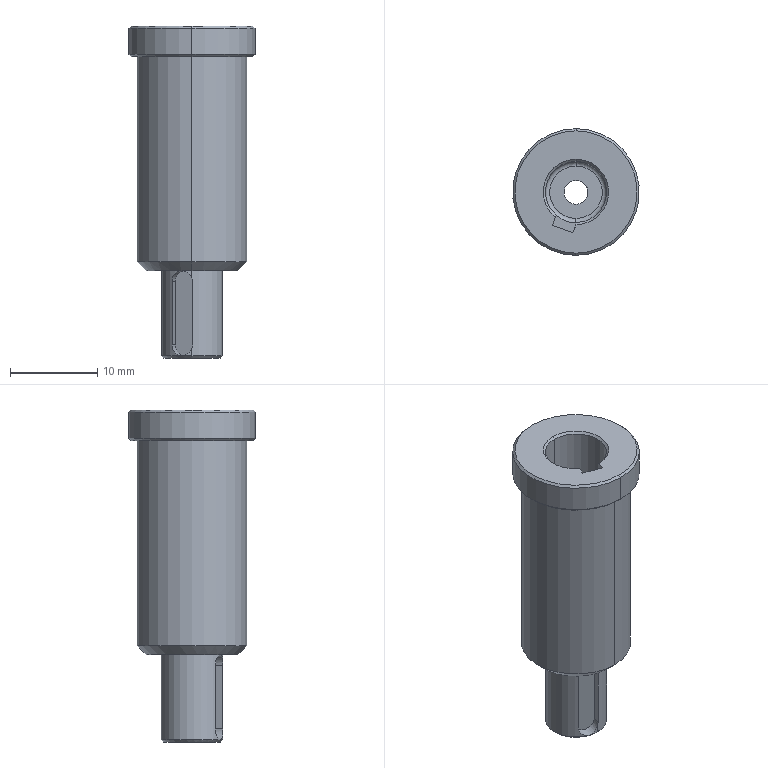Part | STEP file | 2026.6.15-Main Assembly图.sldasm-Part-156 | 1 solid | 41 faces | box 14.5 x 14.5 x 38 mm | volume 3109 mm3 | cylinder 14 | cone 13 | plane 12 | torus 2 | commonest cylinder face diameters 7 x6 2.5 x2 2.75 x2 12.5 x2 14.5 x2
STEP:
#1=CARTESIAN_POINT('',(-1571.41,1398.006,3694.571));
#2=VERTEX_POINT('',#1);
#3=CARTESIAN_POINT('',(-1571.418,1387.506,3694.571));
#4=VERTEX_POINT('',#3);
#5=CARTESIAN_POINT('',(-1571.414,1392.756,3694.571));
#6=DIRECTION('',(0.,0.,-1.));
#7=DIRECTION('',(0.0007664,1.,0.));
#8=AXIS2_PLACEMENT_3D('',#5,#6,#7);
#9=CIRCLE('',#8,5.25);
#10=EDGE_CURVE('',#2,#4,#9,.T.);
#11=ORIENTED_EDGE('',*,*,#10,.F.);
#12=CARTESIAN_POINT('',(-1571.409,1399.006,3695.571));
#13=VERTEX_POINT('',#12);
#14=CARTESIAN_POINT('',(-1571.41,1398.006,3694.571));
#15=DIRECTION('',(0.000542,0.7071,0.7071));
#16=VECTOR('',#15,1000.);
#17=LINE('',#14,#16);
#18=EDGE_CURVE('',#2,#13,#17,.T.);
#19=ORIENTED_EDGE('',*,*,#18,.T.);
#20=CARTESIAN_POINT('',(-1571.419,1386.506,3695.571));
#21=VERTEX_POINT('',#20);
#22=CARTESIAN_POINT('',(-1571.414,1392.756,3695.571));
#23=DIRECTION('',(0.,0.,1.));
#24=DIRECTION('',(0.0007664,1.,0.));
#25=AXIS2_PLACEMENT_3D('',#22,#23,#24);
#26=CIRCLE('',#25,6.25);
#27=EDGE_CURVE('',#21,#13,#26,.T.);
#28=ORIENTED_EDGE('',*,*,#27,.F.);
#29=CARTESIAN_POINT('',(-1571.418,1387.506,3694.571));
#30=DIRECTION('',(-0.000542,-0.7071,0.7071));
#31=VECTOR('',#30,1000.);
#32=LINE('',#29,#31);
#33=EDGE_CURVE('',#4,#21,#32,.T.);
#34=ORIENTED_EDGE('',*,*,#33,.F.);
#35=EDGE_LOOP('',(#11,#19,#28,#34));
#36=FACE_OUTER_BOUND('',#35,.T.);
#37=CARTESIAN_POINT('',(-1571.414,1392.756,3694.571));
#38=DIRECTION('',(0.,0.,1.));
#39=DIRECTION('',(-0.0007664,-1.,0.));
#40=AXIS2_PLACEMENT_3D('',#37,#38,#39);
#41=CONICAL_SURFACE('',#40,5.25,0.7854);
#42=ADVANCED_FACE('',(#36),#41,.T.);
#43=CARTESIAN_POINT('',(-1571.412,1396.006,3684.571));
#44=VERTEX_POINT('',#43);
#45=CARTESIAN_POINT('',(-1571.417,1389.506,3684.571));
#46=VERTEX_POINT('',#45);
#47=CARTESIAN_POINT('',(-1571.414,1392.756,3684.571));
#48=DIRECTION('',(0.,0.,-1.));
#49=DIRECTION('',(0.0007664,1.,0.));
#50=AXIS2_PLACEMENT_3D('',#47,#48,#49);
#51=CIRCLE('',#50,3.25);
#52=EDGE_CURVE('',#44,#46,#51,.T.);
#53=ORIENTED_EDGE('',*,*,#52,.F.);
#54=CARTESIAN_POINT('',(-1571.411,1396.256,3684.821));
#55=VERTEX_POINT('',#54);
#56=CARTESIAN_POINT('',(-1571.412,1396.006,3684.571));
#57=DIRECTION('',(0.000542,0.7071,0.7071));
#58=VECTOR('',#57,1000.);
#59=LINE('',#56,#58);
#60=EDGE_CURVE('',#44,#55,#59,.T.);
#61=ORIENTED_EDGE('',*,*,#60,.T.);
#62=CARTESIAN_POINT('',(-1571.417,1389.256,3684.821));
#63=VERTEX_POINT('',#62);
#64=CARTESIAN_POINT('',(-1571.414,1392.756,3684.821));
#65=DIRECTION('',(0.,0.,1.));
#66=DIRECTION('',(0.0007664,1.,0.));
#67=AXIS2_PLACEMENT_3D('',#64,#65,#66);
#68=CIRCLE('',#67,3.5);
#69=EDGE_CURVE('',#63,#55,#68,.T.);
#70=ORIENTED_EDGE('',*,*,#69,.F.);
#71=CARTESIAN_POINT('',(-1571.417,1389.506,3684.571));
#72=DIRECTION('',(-0.000542,-0.7071,0.7071));
#73=VECTOR('',#72,1000.);
#74=LINE('',#71,#73);
#75=EDGE_CURVE('',#46,#63,#74,.T.);
#76=ORIENTED_EDGE('',*,*,#75,.F.);
#77=EDGE_LOOP('',(#53,#61,#70,#76));
#78=FACE_OUTER_BOUND('',#77,.T.);
#79=CARTESIAN_POINT('',(-1571.414,1392.756,3684.571));
#80=DIRECTION('',(0.,0.,1.));
#81=DIRECTION('',(-0.0007664,-1.,0.));
#82=AXIS2_PLACEMENT_3D('',#79,#80,#81);
#83=CONICAL_SURFACE('',#82,3.25,0.7854);
#84=ADVANCED_FACE('',(#78),#83,.T.);
#85=CARTESIAN_POINT('',(-1571.415,1391.381,3684.821));
#86=VERTEX_POINT('',#85);
#87=CARTESIAN_POINT('',(-1571.413,1394.131,3684.821));
#88=VERTEX_POINT('',#87);
#89=CARTESIAN_POINT('',(-1571.414,1392.756,3684.821));
#90=DIRECTION('',(0.,0.,-1.));
#91=DIRECTION('',(0.0007664,1.,0.));
#92=AXIS2_PLACEMENT_3D('',#89,#90,#91);
#93=CIRCLE('',#92,1.375);
#94=EDGE_CURVE('',#86,#88,#93,.T.);
#95=ORIENTED_EDGE('',*,*,#94,.F.);
#96=CARTESIAN_POINT('',(-1571.415,1391.131,3684.571));
#97=VERTEX_POINT('',#96);
#98=CARTESIAN_POINT('',(-1571.415,1391.131,3684.571));
#99=DIRECTION('',(-0.000542,-0.7071,-0.7071));
#100=VECTOR('',#99,1000.);
#101=LINE('',#98,#100);
#102=EDGE_CURVE('',#86,#97,#101,.T.);
#103=ORIENTED_EDGE('',*,*,#102,.T.);
#104=CARTESIAN_POINT('',(-1571.413,1394.381,3684.571));
#105=VERTEX_POINT('',#104);
#106=CARTESIAN_POINT('',(-1571.414,1392.756,3684.571));
#107=DIRECTION('',(0.,0.,1.));
#108=DIRECTION('',(0.0007664,1.,0.));
#109=AXIS2_PLACEMENT_3D('',#106,#107,#108);
#110=CIRCLE('',#109,1.625);
#111=EDGE_CURVE('',#105,#97,#110,.T.);
#112=ORIENTED_EDGE('',*,*,#111,.F.);
#113=CARTESIAN_POINT('',(-1571.413,1394.381,3684.571));
#114=DIRECTION('',(0.000542,0.7071,-0.7071));
#115=VECTOR('',#114,1000.);
#116=LINE('',#113,#115);
#117=EDGE_CURVE('',#88,#105,#116,.T.);
#118=ORIENTED_EDGE('',*,*,#117,.F.);
#119=EDGE_LOOP('',(#95,#103,#112,#118));
#120=FACE_OUTER_BOUND('',#119,.T.);
#121=CARTESIAN_POINT('',(-1571.414,1392.756,3684.571));
#122=DIRECTION('',(0.,0.,-1.));
#123=DIRECTION('',(0.0007664,1.,0.));
#124=AXIS2_PLACEMENT_3D('',#121,#122,#123);
#125=CONICAL_SURFACE('',#124,1.625,0.7854);
#126=ADVANCED_FACE('',(#120),#125,.F.);
#127=CARTESIAN_POINT('',(-1571.411,1396.256,3722.321));
#128=VERTEX_POINT('',#127);
#129=CARTESIAN_POINT('',(-1573.696,1390.103,3722.321));
#130=VERTEX_POINT('',#129);
#131=CARTESIAN_POINT('',(-1571.414,1392.756,3722.321));
#132=DIRECTION('',(0.,0.,1.));
#133=DIRECTION('',(0.0007664,1.,0.));
#134=AXIS2_PLACEMENT_3D('',#131,#132,#133);
#135=CIRCLE('',#134,3.5);
#136=EDGE_CURVE('',#128,#130,#135,.T.);
#137=ORIENTED_EDGE('',*,*,#136,.F.);
#138=CARTESIAN_POINT('',(-1571.411,1396.506,3722.571));
#139=VERTEX_POINT('',#138);
#140=CARTESIAN_POINT('',(-1571.411,1396.506,3722.571));
#141=DIRECTION('',(0.000542,0.7071,0.7071));
#142=VECTOR('',#141,1000.);
#143=LINE('',#140,#142);
#144=EDGE_CURVE('',#128,#139,#143,.T.);
#145=ORIENTED_EDGE('',*,*,#144,.T.);
#146=CARTESIAN_POINT('',(-1573.787,1389.852,3722.571));
#147=VERTEX_POINT('',#146);
#148=CARTESIAN_POINT('',(-1571.414,1392.756,3722.571));
#149=DIRECTION('',(0.,0.,-1.));
#150=DIRECTION('',(0.0007664,1.,0.));
#151=AXIS2_PLACEMENT_3D('',#148,#149,#150);
#152=CIRCLE('',#151,3.75);
#153=EDGE_CURVE('',#147,#139,#152,.T.);
#154=ORIENTED_EDGE('',*,*,#153,.F.);
#155=CARTESIAN_POINT('',(-1573.696,1390.103,3722.321));
#156=CARTESIAN_POINT('',(-1573.727,1390.019,3722.404));
#157=CARTESIAN_POINT('',(-1573.757,1389.936,3722.487));
#158=CARTESIAN_POINT('',(-1573.787,1389.852,3722.571));
#159=B_SPLINE_CURVE_WITH_KNOTS('',3,(#155,#156,#157,#158),.UNSPECIFIED.,.F.,.F.,(4,4),(0.,0.0003653),.UNSPECIFIED.);
#160=EDGE_CURVE('',#130,#147,#159,.T.);
#161=ORIENTED_EDGE('',*,*,#160,.F.);
#162=EDGE_LOOP('',(#137,#145,#154,#161));
#163=FACE_OUTER_BOUND('',#162,.T.);
#164=CARTESIAN_POINT('',(-1571.414,1392.756,3722.571));
#165=DIRECTION('',(0.,0.,1.));
#166=DIRECTION('',(-0.0007664,-1.,0.));
#167=AXIS2_PLACEMENT_3D('',#164,#165,#166);
#168=CONICAL_SURFACE('',#167,3.75,0.7854);
#169=ADVANCED_FACE('',(#163),#168,.F.);
#170=ORIENTED_EDGE('',*,*,#144,.F.);
#171=CARTESIAN_POINT('',(-1571.344,1389.257,3722.321));
#172=VERTEX_POINT('',#171);
#173=CARTESIAN_POINT('',(-1571.414,1392.756,3722.321));
#174=DIRECTION('',(0.,0.,1.));
#175=DIRECTION('',(0.0007664,1.,0.));
#176=AXIS2_PLACEMENT_3D('',#173,#174,#175);
#177=CIRCLE('',#176,3.5);
#178=EDGE_CURVE('',#172,#128,#177,.T.);
#179=ORIENTED_EDGE('',*,*,#178,.F.);
#180=CARTESIAN_POINT('',(-1571.417,1389.054,3722.524));
#181=VERTEX_POINT('',#180);
#182=CARTESIAN_POINT('',(-1571.417,1389.054,3722.524));
#183=CARTESIAN_POINT('',(-1571.393,1389.121,3722.456));
#184=CARTESIAN_POINT('',(-1571.368,1389.189,3722.388));
#185=CARTESIAN_POINT('',(-1571.344,1389.257,3722.321));
#186=B_SPLINE_CURVE_WITH_KNOTS('',3,(#182,#183,#184,#185),.UNSPECIFIED.,.F.,.F.,(4,4),(0.00006889,0.0003653),.UNSPECIFIED.);
#187=EDGE_CURVE('',#181,#172,#186,.T.);
#188=ORIENTED_EDGE('',*,*,#187,.F.);
#189=CARTESIAN_POINT('',(-1571.417,1389.006,3722.571));
#190=VERTEX_POINT('',#189);
#191=CARTESIAN_POINT('',(-1571.417,1389.006,3722.571));
#192=DIRECTION('',(-0.000542,-0.7071,0.7071));
#193=VECTOR('',#192,1000.);
#194=LINE('',#191,#193);
#195=EDGE_CURVE('',#181,#190,#194,.T.);
#196=ORIENTED_EDGE('',*,*,#195,.T.);
#197=CARTESIAN_POINT('',(-1571.414,1392.756,3722.571));
#198=DIRECTION('',(0.,0.,-1.));
#199=DIRECTION('',(0.0007664,1.,0.));
#200=AXIS2_PLACEMENT_3D('',#197,#198,#199);
#201=CIRCLE('',#200,3.75);
#202=EDGE_CURVE('',#139,#190,#201,.T.);
#203=ORIENTED_EDGE('',*,*,#202,.F.);
#204=EDGE_LOOP('',(#170,#179,#188,#196,#203));
#205=FACE_OUTER_BOUND('',#204,.T.);
#206=CARTESIAN_POINT('',(-1571.414,1392.756,3722.571));
#207=DIRECTION('',(0.,0.,1.));
#208=DIRECTION('',(-0.0007664,-1.,0.));
#209=AXIS2_PLACEMENT_3D('',#206,#207,#208);
#210=CONICAL_SURFACE('',#209,3.75,0.7854);
#211=ADVANCED_FACE('',(#205),#210,.F.);
#212=CARTESIAN_POINT('',(-1571.419,1385.756,3722.571));
#213=VERTEX_POINT('',#212);
#214=CARTESIAN_POINT('',(-1571.409,1399.756,3722.571));
#215=VERTEX_POINT('',#214);
#216=CARTESIAN_POINT('',(-1571.414,1392.756,3722.571));
#217=DIRECTION('',(0.,0.,1.));
#218=DIRECTION('',(0.0007664,1.,0.));
#219=AXIS2_PLACEMENT_3D('',#216,#217,#218);
#220=CIRCLE('',#219,7.);
#221=EDGE_CURVE('',#213,#215,#220,.T.);
#222=ORIENTED_EDGE('',*,*,#221,.F.);
#223=CARTESIAN_POINT('',(-1571.42,1385.506,3722.321));
#224=VERTEX_POINT('',#223);
#225=CARTESIAN_POINT('',(-1571.42,1385.506,3722.321));
#226=DIRECTION('',(-0.000542,-0.7071,-0.7071));
#227=VECTOR('',#226,1000.);
#228=LINE('',#225,#227);
#229=EDGE_CURVE('',#213,#224,#228,.T.);
#230=ORIENTED_EDGE('',*,*,#229,.T.);
#231=CARTESIAN_POINT('',(-1571.409,1400.006,3722.321));
#232=VERTEX_POINT('',#231);
#233=CARTESIAN_POINT('',(-1571.414,1392.756,3722.321));
#234=DIRECTION('',(0.,0.,-1.));
#235=DIRECTION('',(0.0007664,1.,0.));
#236=AXIS2_PLACEMENT_3D('',#233,#234,#235);
#237=CIRCLE('',#236,7.25);
#238=EDGE_CURVE('',#232,#224,#237,.T.);
#239=ORIENTED_EDGE('',*,*,#238,.F.);
#240=CARTESIAN_POINT('',(-1571.409,1400.006,3722.321));
#241=DIRECTION('',(0.000542,0.7071,-0.7071));
#242=VECTOR('',#241,1000.);
#243=LINE('',#240,#242);
#244=EDGE_CURVE('',#215,#232,#243,.T.);
#245=ORIENTED_EDGE('',*,*,#244,.F.);
#246=EDGE_LOOP('',(#222,#230,#239,#245));
#247=FACE_OUTER_BOUND('',#246,.T.);
#248=CARTESIAN_POINT('',(-1571.414,1392.756,3722.321));
#249=DIRECTION('',(0.,0.,-1.));
#250=DIRECTION('',(0.0007664,1.,0.));
#251=AXIS2_PLACEMENT_3D('',#248,#249,#250);
#252=CONICAL_SURFACE('',#251,7.25,0.7854);
#253=ADVANCED_FACE('',(#247),#252,.T.);
#254=CARTESIAN_POINT('',(-1571.409,1399.756,3719.071));
#255=VERTEX_POINT('',#254);
#256=CARTESIAN_POINT('',(-1571.419,1385.756,3719.071));
#257=VERTEX_POINT('',#256);
#258=CARTESIAN_POINT('',(-1571.414,1392.756,3719.071));
#259=DIRECTION('',(0.,0.,-1.));
#260=DIRECTION('',(0.0007664,1.,0.));
#261=AXIS2_PLACEMENT_3D('',#258,#259,#260);
#262=CIRCLE('',#261,7.);
#263=EDGE_CURVE('',#255,#257,#262,.T.);
#264=ORIENTED_EDGE('',*,*,#263,.F.);
#265=CARTESIAN_POINT('',(-1571.409,1400.006,3719.321));
#266=VERTEX_POINT('',#265);
#267=CARTESIAN_POINT('',(-1571.409,1399.756,3719.071));
#268=DIRECTION('',(0.000542,0.7071,0.7071));
#269=VECTOR('',#268,1000.);
#270=LINE('',#267,#269);
#271=EDGE_CURVE('',#255,#266,#270,.T.);
#272=ORIENTED_EDGE('',*,*,#271,.T.);
#273=CARTESIAN_POINT('',(-1571.42,1385.506,3719.321));
#274=VERTEX_POINT('',#273);
#275=CARTESIAN_POINT('',(-1571.414,1392.756,3719.321));
#276=DIRECTION('',(0.,0.,1.));
#277=DIRECTION('',(0.0007664,1.,0.));
#278=AXIS2_PLACEMENT_3D('',#275,#276,#277);
#279=CIRCLE('',#278,7.25);
#280=EDGE_CURVE('',#274,#266,#279,.T.);
#281=ORIENTED_EDGE('',*,*,#280,.F.);
#282=CARTESIAN_POINT('',(-1571.419,1385.756,3719.071));
#283=DIRECTION('',(-0.000542,-0.7071,0.7071));
#284=VECTOR('',#283,1000.);
#285=LINE('',#282,#284);
#286=EDGE_CURVE('',#257,#274,#285,.T.);
#287=ORIENTED_EDGE('',*,*,#286,.F.);
#288=EDGE_LOOP('',(#264,#272,#281,#287));
#289=FACE_OUTER_BOUND('',#288,.T.);
#290=CARTESIAN_POINT('',(-1571.414,1392.756,3719.071));
#291=DIRECTION('',(0.,0.,1.));
#292=DIRECTION('',(-0.0007664,-1.,0.));
#293=AXIS2_PLACEMENT_3D('',#290,#291,#292);
#294=CONICAL_SURFACE('',#293,7.,0.7854);
#295=ADVANCED_FACE('',(#289),#294,.T.);
#296=CARTESIAN_POINT('',(-1571.417,1389.256,3706.321));
#297=VERTEX_POINT('',#296);
#298=CARTESIAN_POINT('',(-1571.411,1396.256,3706.321));
#299=VERTEX_POINT('',#298);
#300=CARTESIAN_POINT('',(-1571.414,1392.756,3706.321));
#301=DIRECTION('',(0.,0.,-1.));
#302=DIRECTION('',(0.0007664,1.,0.));
#303=AXIS2_PLACEMENT_3D('',#300,#301,#302);
#304=CIRCLE('',#303,3.5);
#305=EDGE_CURVE('',#297,#299,#304,.T.);
#306=ORIENTED_EDGE('',*,*,#305,.F.);
#307=CARTESIAN_POINT('',(-1571.416,1389.756,3705.821));
#308=VERTEX_POINT('',#307);
#309=CARTESIAN_POINT('',(-1571.416,1389.756,3706.321));
#310=DIRECTION('',(1.,-0.0007664,0.));
#311=DIRECTION('',(0.0007664,1.,0.));
#312=AXIS2_PLACEMENT_3D('',#309,#310,#311);
#313=CIRCLE('',#312,0.5);
#314=EDGE_CURVE('',#297,#308,#313,.T.);
#315=ORIENTED_EDGE('',*,*,#314,.T.);
#316=CARTESIAN_POINT('',(-1571.412,1395.756,3705.821));
#317=VERTEX_POINT('',#316);
#318=CARTESIAN_POINT('',(-1571.414,1392.756,3705.821));
#319=DIRECTION('',(0.,0.,1.));
#320=DIRECTION('',(0.0007664,1.,0.));
#321=AXIS2_PLACEMENT_3D('',#318,#319,#320);
#322=CIRCLE('',#321,3.);
#323=EDGE_CURVE('',#317,#308,#322,.T.);
#324=ORIENTED_EDGE('',*,*,#323,.F.);
#325=CARTESIAN_POINT('',(-1571.412,1395.756,3706.321));
#326=DIRECTION('',(-1.,0.0007664,0.));
#327=DIRECTION('',(-0.0007664,-1.,0.));
#328=AXIS2_PLACEMENT_3D('',#325,#326,#327);
#329=CIRCLE('',#328,0.5);
#330=EDGE_CURVE('',#299,#317,#329,.T.);
#331=ORIENTED_EDGE('',*,*,#330,.F.);
#332=EDGE_LOOP('',(#306,#315,#324,#331));
#333=FACE_OUTER_BOUND('',#332,.T.);
#334=CARTESIAN_POINT('',(-1571.414,1392.756,3706.321));
#335=DIRECTION('',(0.,0.,-1.));
#336=DIRECTION('',(0.0007664,1.,0.));
#337=AXIS2_PLACEMENT_3D('',#334,#335,#336);
#338=TOROIDAL_SURFACE('',#337,3.,0.5);
#339=ADVANCED_FACE('',(#333),#338,.F.);
#340=ORIENTED_EDGE('',*,*,#94,.T.);
#341=CARTESIAN_POINT('',(-1571.413,1394.131,3705.821));
#342=VERTEX_POINT('',#341);
#343=CARTESIAN_POINT('',(-1571.413,1394.131,3684.571));
#344=DIRECTION('',(0.,0.,1.));
#345=VECTOR('',#344,1000.);
#346=LINE('',#343,#345);
#347=EDGE_CURVE('',#88,#342,#346,.T.);
#348=ORIENTED_EDGE('',*,*,#347,.T.);
#349=CARTESIAN_POINT('',(-1571.415,1391.381,3705.821));
#350=VERTEX_POINT('',#349);
#351=CARTESIAN_POINT('',(-1571.414,1392.756,3705.821));
#352=DIRECTION('',(0.,0.,1.));
#353=DIRECTION('',(0.0007664,1.,0.));
#354=AXIS2_PLACEMENT_3D('',#351,#352,#353);
#355=CIRCLE('',#354,1.375);
#356=EDGE_CURVE('',#342,#350,#355,.T.);
#357=ORIENTED_EDGE('',*,*,#356,.T.);
#358=CARTESIAN_POINT('',(-1571.415,1391.381,3684.571));
#359=DIRECTION('',(0.,0.,1.));
#360=VECTOR('',#359,1000.);
#361=LINE('',#358,#360);
#362=EDGE_CURVE('',#86,#350,#361,.T.);
#363=ORIENTED_EDGE('',*,*,#362,.F.);
#364=EDGE_LOOP('',(#340,#348,#357,#363));
#365=FACE_OUTER_BOUND('',#364,.T.);
#366=CARTESIAN_POINT('',(-1571.414,1392.756,3684.571));
#367=DIRECTION('',(0.,0.,1.));
#368=DIRECTION('',(-0.0007664,-1.,0.));
#369=AXIS2_PLACEMENT_3D('',#366,#367,#368);
#370=CYLINDRICAL_SURFACE('',#369,1.375);
#371=ADVANCED_FACE('',(#365),#370,.F.);
#372=ORIENTED_EDGE('',*,*,#27,.T.);
#373=CARTESIAN_POINT('',(-1571.409,1399.006,3719.071));
#374=VERTEX_POINT('',#373);
#375=CARTESIAN_POINT('',(-1571.409,1399.006,3694.571));
#376=DIRECTION('',(0.,0.,1.));
#377=VECTOR('',#376,1000.);
#378=LINE('',#375,#377);
#379=EDGE_CURVE('',#13,#374,#378,.T.);
#380=ORIENTED_EDGE('',*,*,#379,.T.);
#381=CARTESIAN_POINT('',(-1571.419,1386.506,3719.071));
#382=VERTEX_POINT('',#381);
#383=CARTESIAN_POINT('',(-1571.414,1392.756,3719.071));
#384=DIRECTION('',(0.,0.,1.));
#385=DIRECTION('',(0.0007664,1.,0.));
#386=AXIS2_PLACEMENT_3D('',#383,#384,#385);
#387=CIRCLE('',#386,6.25);
#388=EDGE_CURVE('',#382,#374,#387,.T.);
#389=ORIENTED_EDGE('',*,*,#388,.F.);
#390=CARTESIAN_POINT('',(-1571.419,1386.506,3694.571));
#391=DIRECTION('',(0.,0.,1.));
#392=VECTOR('',#391,1000.);
#393=LINE('',#390,#392);
#394=EDGE_CURVE('',#21,#382,#393,.T.);
#395=ORIENTED_EDGE('',*,*,#394,.F.);
#396=EDGE_LOOP('',(#372,#380,#389,#395));
#397=FACE_OUTER_BOUND('',#396,.T.);
#398=CARTESIAN_POINT('',(-1571.414,1392.756,3694.571));
#399=DIRECTION('',(0.,0.,1.));
#400=DIRECTION('',(-0.0007664,-1.,0.));
#401=AXIS2_PLACEMENT_3D('',#398,#399,#400);
#402=CYLINDRICAL_SURFACE('',#401,6.25);
#403=ADVANCED_FACE('',(#397),#402,.T.);
#404=ORIENTED_EDGE('',*,*,#280,.T.);
#405=CARTESIAN_POINT('',(-1571.409,1400.006,3719.071));
#406=DIRECTION('',(0.,0.,1.));
#407=VECTOR('',#406,1000.);
#408=LINE('',#405,#407);
#409=EDGE_CURVE('',#266,#232,#408,.T.);
#410=ORIENTED_EDGE('',*,*,#409,.T.);
#411=ORIENTED_EDGE('',*,*,#238,.T.);
#412=CARTESIAN_POINT('',(-1571.42,1385.506,3719.071));
#413=DIRECTION('',(0.,0.,1.));
#414=VECTOR('',#413,1000.);
#415=LINE('',#412,#414);
#416=EDGE_CURVE('',#274,#224,#415,.T.);
#417=ORIENTED_EDGE('',*,*,#416,.F.);
#418=EDGE_LOOP('',(#404,#410,#411,#417));
#419=FACE_OUTER_BOUND('',#418,.T.);
#420=CARTESIAN_POINT('',(-1571.414,1392.756,3719.071));
#421=DIRECTION('',(0.,0.,1.));
#422=DIRECTION('',(-0.0007664,-1.,0.));
#423=AXIS2_PLACEMENT_3D('',#420,#421,#422);
#424=CYLINDRICAL_SURFACE('',#423,7.25);
#425=ADVANCED_FACE('',(#419),#424,.T.);
#426=ORIENTED_EDGE('',*,*,#69,.T.);
#427=CARTESIAN_POINT('',(-1571.411,1396.256,3694.571));
#428=VERTEX_POINT('',#427);
#429=CARTESIAN_POINT('',(-1571.411,1396.256,3684.571));
#430=DIRECTION('',(0.,0.,1.));
#431=VECTOR('',#430,1000.);
#432=LINE('',#429,#431);
#433=EDGE_CURVE('',#55,#428,#432,.T.);
#434=ORIENTED_EDGE('',*,*,#433,.T.);
#435=CARTESIAN_POINT('',(-1571.417,1389.256,3694.571));
#436=VERTEX_POINT('',#435);
#437=CARTESIAN_POINT('',(-1571.414,1392.756,3694.571));
#438=DIRECTION('',(0.,0.,-1.));
#439=DIRECTION('',(0.0007664,1.,0.));
#440=AXIS2_PLACEMENT_3D('',#437,#438,#439);
#441=CIRCLE('',#440,3.5);
#442=EDGE_CURVE('',#428,#436,#441,.T.);
#443=ORIENTED_EDGE('',*,*,#442,.T.);
#444=CARTESIAN_POINT('',(-1571.417,1389.256,3693.729));
#445=VERTEX_POINT('',#444);
#446=CARTESIAN_POINT('',(-1571.417,1389.256,3684.571));
#447=DIRECTION('',(0.,0.,1.));
#448=VECTOR('',#447,1000.);
#449=LINE('',#446,#448);
#450=EDGE_CURVE('',#445,#436,#449,.T.);
#451=ORIENTED_EDGE('',*,*,#450,.F.);
#452=CARTESIAN_POINT('',(-1571.344,1389.257,3693.321));
#453=VERTEX_POINT('',#452);
#454=CARTESIAN_POINT('',(-1571.417,1389.256,3693.729));
#455=CARTESIAN_POINT('',(-1571.369,1389.256,3693.6));
#456=CARTESIAN_POINT('',(-1571.344,1389.257,3693.461));
#457=CARTESIAN_POINT('',(-1571.344,1389.257,3693.321));
#458=B_SPLINE_CURVE_WITH_KNOTS('',3,(#454,#455,#456,#457),.UNSPECIFIED.,.F.,.F.,(4,4),(0.003526,0.003939),.UNSPECIFIED.);
#459=EDGE_CURVE('',#445,#453,#458,.T.);
#460=ORIENTED_EDGE('',*,*,#459,.T.);
#461=CARTESIAN_POINT('',(-1571.344,1389.257,3686.071));
#462=VERTEX_POINT('',#461);
#463=CARTESIAN_POINT('',(-1571.344,1389.257,3684.571));
#464=DIRECTION('',(0.,0.,-1.));
#465=VECTOR('',#464,1000.);
#466=LINE('',#463,#465);
#467=EDGE_CURVE('',#453,#462,#466,.T.);
#468=ORIENTED_EDGE('',*,*,#467,.T.);
#469=CARTESIAN_POINT('',(-1571.417,1389.256,3685.663));
#470=VERTEX_POINT('',#469);
#471=CARTESIAN_POINT('',(-1571.344,1389.257,3686.071));
#472=CARTESIAN_POINT('',(-1571.344,1389.257,3685.931));
#473=CARTESIAN_POINT('',(-1571.369,1389.256,3685.794));
#474=CARTESIAN_POINT('',(-1571.417,1389.256,3685.663));
#475=B_SPLINE_CURVE_WITH_KNOTS('',3,(#471,#472,#473,#474),.UNSPECIFIED.,.F.,.F.,(4,4),(0.,0.0004145),.UNSPECIFIED.);
#476=EDGE_CURVE('',#462,#470,#475,.T.);
#477=ORIENTED_EDGE('',*,*,#476,.T.);
#478=CARTESIAN_POINT('',(-1571.417,1389.256,3684.571));
#479=DIRECTION('',(0.,0.,1.));
#480=VECTOR('',#479,1000.);
#481=LINE('',#478,#480);
#482=EDGE_CURVE('',#63,#470,#481,.T.);
#483=ORIENTED_EDGE('',*,*,#482,.F.);
#484=EDGE_LOOP('',(#426,#434,#443,#451,#460,#468,#477,#483));
#485=FACE_OUTER_BOUND('',#484,.T.);
#486=CARTESIAN_POINT('',(-1571.414,1392.756,3684.571));
#487=DIRECTION('',(0.,0.,1.));
#488=DIRECTION('',(-0.0007664,-1.,0.));
#489=AXIS2_PLACEMENT_3D('',#486,#487,#488);
#490=CYLINDRICAL_SURFACE('',#489,3.5);
#491=ADVANCED_FACE('',(#485),#490,.T.);
#492=CARTESIAN_POINT('',(-1572.598,1389.463,3684.821));
#493=VERTEX_POINT('',#492);
#494=CARTESIAN_POINT('',(-1571.414,1392.756,3684.821));
#495=DIRECTION('',(0.,0.,1.));
#496=DIRECTION('',(0.0007664,1.,0.));
#497=AXIS2_PLACEMENT_3D('',#494,#495,#496);
#498=CIRCLE('',#497,3.5);
#499=EDGE_CURVE('',#493,#63,#498,.T.);
#500=ORIENTED_EDGE('',*,*,#499,.T.);
#501=ORIENTED_EDGE('',*,*,#482,.T.);
#502=CARTESIAN_POINT('',(-1571.417,1389.256,3685.663));
#503=CARTESIAN_POINT('',(-1571.507,1389.256,3685.416));
#504=CARTESIAN_POINT('',(-1571.675,1389.259,3685.205));
#505=CARTESIAN_POINT('',(-1571.994,1389.303,3684.979));
#506=CARTESIAN_POINT('',(-1572.109,1389.324,3684.921));
#507=CARTESIAN_POINT('',(-1572.351,1389.382,3684.841));
#508=CARTESIAN_POINT('',(-1572.476,1389.419,3684.821));
#509=CARTESIAN_POINT('',(-1572.598,1389.463,3684.821));
#510=B_SPLINE_CURVE_WITH_KNOTS('',3,(#502,#503,#504,#505,#506,#507,#508,#509),.UNSPECIFIED.,.F.,.F.,(4,2,2,4),(0.0004145,0.001193,0.001582,0.001971),.UNSPECIFIED.);
#511=EDGE_CURVE('',#470,#493,#510,.T.);
#512=ORIENTED_EDGE('',*,*,#511,.T.);
#513=EDGE_LOOP('',(#500,#501,#512));
#514=FACE_OUTER_BOUND('',#513,.T.);
#515=CARTESIAN_POINT('',(-1571.414,1392.756,3684.571));
#516=DIRECTION('',(0.,0.,1.));
#517=DIRECTION('',(-0.0007664,-1.,0.));
#518=AXIS2_PLACEMENT_3D('',#515,#516,#517);
#519=CYLINDRICAL_SURFACE('',#518,3.5);
#520=ADVANCED_FACE('',(#514),#519,.T.);
#521=CARTESIAN_POINT('',(-1572.598,1389.463,3694.571));
#522=VERTEX_POINT('',#521);
#523=CARTESIAN_POINT('',(-1572.598,1389.463,3694.571));
#524=CARTESIAN_POINT('',(-1572.476,1389.419,3694.571));
#525=CARTESIAN_POINT('',(-1572.35,1389.382,3694.55));
#526=CARTESIAN_POINT('',(-1572.109,1389.324,3694.471));
#527=CARTESIAN_POINT('',(-1571.993,1389.303,3694.411));
#528=CARTESIAN_POINT('',(-1571.676,1389.26,3694.188));
#529=CARTESIAN_POINT('',(-1571.506,1389.256,3693.972));
#530=CARTESIAN_POINT('',(-1571.417,1389.256,3693.729));
#531=B_SPLINE_CURVE_WITH_KNOTS('',3,(#523,#524,#525,#526,#527,#528,#529,#530),.UNSPECIFIED.,.F.,.F.,(4,2,2,4),(0.001971,0.00236,0.002749,0.003526),.UNSPECIFIED.);
#532=EDGE_CURVE('',#522,#445,#531,.T.);
#533=ORIENTED_EDGE('',*,*,#532,.T.);
#534=ORIENTED_EDGE('',*,*,#450,.T.);
#535=CARTESIAN_POINT('',(-1571.414,1392.756,3694.571));
#536=DIRECTION('',(0.,0.,-1.));
#537=DIRECTION('',(0.0007664,1.,0.));
#538=AXIS2_PLACEMENT_3D('',#535,#536,#537);
#539=CIRCLE('',#538,3.5);
#540=EDGE_CURVE('',#436,#522,#539,.T.);
#541=ORIENTED_EDGE('',*,*,#540,.T.);
#542=EDGE_LOOP('',(#533,#534,#541));
#543=FACE_OUTER_BOUND('',#542,.T.);
#544=CARTESIAN_POINT('',(-1571.414,1392.756,3684.571));
#545=DIRECTION('',(0.,0.,1.));
#546=DIRECTION('',(-0.0007664,-1.,0.));
#547=AXIS2_PLACEMENT_3D('',#544,#545,#546);
#548=CYLINDRICAL_SURFACE('',#547,3.5);
#549=ADVANCED_FACE('',(#543),#548,.T.);
#550=ORIENTED_EDGE('',*,*,#305,.T.);
#551=CARTESIAN_POINT('',(-1571.411,1396.256,3705.821));
#552=DIRECTION('',(0.,0.,1.));
#553=VECTOR('',#552,1000.);
#554=LINE('',#551,#553);
#555=EDGE_CURVE('',#299,#128,#554,.T.);
#556=ORIENTED_EDGE('',*,*,#555,.T.);
#557=ORIENTED_EDGE('',*,*,#136,.T.);
#558=CARTESIAN_POINT('',(-1573.696,1390.103,3707.571));
#559=VERTEX_POINT('',#558);
#560=CARTESIAN_POINT('',(-1573.696,1390.103,3707.571));
#561=DIRECTION('',(0.,0.,1.));
#562=VECTOR('',#561,1000.);
#563=LINE('',#560,#562);
#564=EDGE_CURVE('',#559,#130,#563,.T.);
#565=ORIENTED_EDGE('',*,*,#564,.F.);
#566=CARTESIAN_POINT('',(-1571.417,1389.256,3707.571));
#567=VERTEX_POINT('',#566);
#568=CARTESIAN_POINT('',(-1571.414,1392.756,3707.571));
#569=DIRECTION('',(0.,0.,-1.));
#570=DIRECTION('',(-0.0007664,-1.,0.));
#571=AXIS2_PLACEMENT_3D('',#568,#569,#570);
#572=CIRCLE('',#571,3.5);
#573=EDGE_CURVE('',#567,#559,#572,.T.);
#574=ORIENTED_EDGE('',*,*,#573,.F.);
#575=CARTESIAN_POINT('',(-1571.417,1389.256,3705.821));
#576=DIRECTION('',(0.,0.,1.));
#577=VECTOR('',#576,1000.);
#578=LINE('',#575,#577);
#579=EDGE_CURVE('',#297,#567,#578,.T.);
#580=ORIENTED_EDGE('',*,*,#579,.F.);
#581=EDGE_LOOP('',(#550,#556,#557,#565,#574,#580));
#582=FACE_OUTER_BOUND('',#581,.T.);
#583=CARTESIAN_POINT('',(-1571.414,1392.756,3705.821));
#584=DIRECTION('',(0.,0.,1.));
#585=DIRECTION('',(-0.0007664,-1.,0.));
#586=AXIS2_PLACEMENT_3D('',#583,#584,#585);
#587=CYLINDRICAL_SURFACE('',#586,3.5);
#588=ADVANCED_FACE('',(#582),#587,.F.);
#589=ORIENTED_EDGE('',*,*,#555,.F.);
#590=CARTESIAN_POINT('',(-1571.414,1392.756,3706.321));
#591=DIRECTION('',(0.,0.,-1.));
#592=DIRECTION('',(0.0007664,1.,0.));
#593=AXIS2_PLACEMENT_3D('',#590,#591,#592);
#594=CIRCLE('',#593,3.5);
#595=EDGE_CURVE('',#299,#297,#594,.T.);
#596=ORIENTED_EDGE('',*,*,#595,.T.);
#597=ORIENTED_EDGE('',*,*,#579,.T.);
#598=CARTESIAN_POINT('',(-1571.344,1389.257,3707.571));
#599=VERTEX_POINT('',#598);
#600=CARTESIAN_POINT('',(-1571.414,1392.756,3707.571));
#601=DIRECTION('',(0.,0.,-1.));
#602=DIRECTION('',(-0.0007664,-1.,0.));
#603=AXIS2_PLACEMENT_3D('',#600,#601,#602);
#604=CIRCLE('',#603,3.5);
#605=EDGE_CURVE('',#599,#567,#604,.T.);
#606=ORIENTED_EDGE('',*,*,#605,.F.);
#607=CARTESIAN_POINT('',(-1571.344,1389.257,3707.571));
#608=DIRECTION('',(0.,0.,1.));
#609=VECTOR('',#608,1000.);
#610=LINE('',#607,#609);
#611=EDGE_CURVE('',#599,#172,#610,.T.);
#612=ORIENTED_EDGE('',*,*,#611,.T.);
#613=ORIENTED_EDGE('',*,*,#178,.T.);
#614=EDGE_LOOP('',(#589,#596,#597,#606,#612,#613));
#615=FACE_OUTER_BOUND('',#614,.T.);
#616=CARTESIAN_POINT('',(-1571.414,1392.756,3705.821));
#617=DIRECTION('',(0.,0.,1.));
#618=DIRECTION('',(-0.0007664,-1.,0.));
#619=AXIS2_PLACEMENT_3D('',#616,#617,#618);
#620=CYLINDRICAL_SURFACE('',#619,3.5);
#621=ADVANCED_FACE('',(#615),#620,.F.);
#622=ORIENTED_EDGE('',*,*,#433,.F.);
#623=CARTESIAN_POINT('',(-1571.414,1392.756,3684.821));
#624=DIRECTION('',(0.,0.,1.));
#625=DIRECTION('',(0.0007664,1.,0.));
#626=AXIS2_PLACEMENT_3D('',#623,#624,#625);
#627=CIRCLE('',#626,3.5);
#628=EDGE_CURVE('',#55,#493,#627,.T.);
#629=ORIENTED_EDGE('',*,*,#628,.T.);
#630=CARTESIAN_POINT('',(-1573.696,1390.103,3686.071));
#631=VERTEX_POINT('',#630);
#632=CARTESIAN_POINT('',(-1572.598,1389.463,3684.821));
#633=CARTESIAN_POINT('',(-1572.676,1389.491,3684.821));
#634=CARTESIAN_POINT('',(-1572.753,1389.522,3684.829));
#635=CARTESIAN_POINT('',(-1572.901,1389.587,3684.861));
#636=CARTESIAN_POINT('',(-1572.971,1389.621,3684.885));
#637=CARTESIAN_POINT('',(-1573.175,1389.728,3684.98));
#638=CARTESIAN_POINT('',(-1573.294,1389.802,3685.072));
#639=CARTESIAN_POINT('',(-1573.441,1389.902,3685.245));
#640=CARTESIAN_POINT('',(-1573.484,1389.934,3685.307));
#641=CARTESIAN_POINT('',(-1573.56,1389.991,3685.442));
#642=CARTESIAN_POINT('',(-1573.592,1390.016,3685.515));
#643=CARTESIAN_POINT('',(-1573.669,1390.079,3685.74));
#644=CARTESIAN_POINT('',(-1573.696,1390.103,3685.904));
#645=CARTESIAN_POINT('',(-1573.696,1390.103,3686.071));
#646=B_SPLINE_CURVE_WITH_KNOTS('',3,(#632,#633,#634,#635,#636,#637,#638,#639,#640,#641,#642,#643,#644,#645),.UNSPECIFIED.,.F.,.F.,(4,2,2,2,2,2,4),(0.001971,0.002217,0.002463,0.002955,0.003201,0.003447,0.003939),.UNSPECIFIED.);
#647=EDGE_CURVE('',#493,#631,#646,.T.);
#648=ORIENTED_EDGE('',*,*,#647,.T.);
#649=CARTESIAN_POINT('',(-1573.696,1390.103,3693.321));
#650=VERTEX_POINT('',#649);
#651=CARTESIAN_POINT('',(-1573.696,1390.103,3684.571));
#652=DIRECTION('',(0.,0.,1.));
#653=VECTOR('',#652,1000.);
#654=LINE('',#651,#653);
#655=EDGE_CURVE('',#631,#650,#654,.T.);
#656=ORIENTED_EDGE('',*,*,#655,.T.);
#657=CARTESIAN_POINT('',(-1573.696,1390.103,3693.321));
#658=CARTESIAN_POINT('',(-1573.696,1390.103,3693.487));
#659=CARTESIAN_POINT('',(-1573.67,1390.079,3693.651));
#660=CARTESIAN_POINT('',(-1573.566,1389.995,3693.953));
#661=CARTESIAN_POINT('',(-1573.489,1389.935,3694.091));
#662=CARTESIAN_POINT('',(-1573.294,1389.802,3694.319));
#663=CARTESIAN_POINT('',(-1573.174,1389.727,3694.412));
#664=CARTESIAN_POINT('',(-1572.905,1389.586,3694.537));
#665=CARTESIAN_POINT('',(-1572.753,1389.518,3694.571));
#666=CARTESIAN_POINT('',(-1572.598,1389.463,3694.571));
#667=B_SPLINE_CURVE_WITH_KNOTS('',3,(#657,#658,#659,#660,#661,#662,#663,#664,#665,#666),.UNSPECIFIED.,.F.,.F.,(4,2,2,2,4),(0.,0.0004927,0.0009855,0.001478,0.001971),.UNSPECIFIED.);
#668=EDGE_CURVE('',#650,#522,#667,.T.);
#669=ORIENTED_EDGE('',*,*,#668,.T.);
#670=CARTESIAN_POINT('',(-1571.414,1392.756,3694.571));
#671=DIRECTION('',(0.,0.,-1.));
#672=DIRECTION('',(0.0007664,1.,0.));
#673=AXIS2_PLACEMENT_3D('',#670,#671,#672);
#674=CIRCLE('',#673,3.5);
#675=EDGE_CURVE('',#522,#428,#674,.T.);
#676=ORIENTED_EDGE('',*,*,#675,.T.);
#677=EDGE_LOOP('',(#622,#629,#648,#656,#669,#676));
#678=FACE_OUTER_BOUND('',#677,.T.);
#679=CARTESIAN_POINT('',(-1571.414,1392.756,3684.571));
#680=DIRECTION('',(0.,0.,1.));
#681=DIRECTION('',(-0.0007664,-1.,0.));
#682=AXIS2_PLACEMENT_3D('',#679,#680,#681);
#683=CYLINDRICAL_SURFACE('',#682,3.5);
#684=ADVANCED_FACE('',(#678),#683,.T.);
#685=ORIENTED_EDGE('',*,*,#111,.T.);
#686=CARTESIAN_POINT('',(-1571.414,1392.756,3684.571));
#687=DIRECTION('',(0.,0.,1.));
#688=DIRECTION('',(0.0007664,1.,0.));
#689=AXIS2_PLACEMENT_3D('',#686,#687,#688);
#690=CIRCLE('',#689,1.625);
#691=EDGE_CURVE('',#97,#105,#690,.T.);
#692=ORIENTED_EDGE('',*,*,#691,.T.);
#693=EDGE_LOOP('',(#685,#692));
#694=FACE_BOUND('',#693,.T.);
#695=CARTESIAN_POINT('',(-1571.414,1392.756,3684.571));
#696=DIRECTION('',(0.,0.,-1.));
#697=DIRECTION('',(0.0007664,1.,0.));
#698=AXIS2_PLACEMENT_3D('',#695,#696,#697);
#699=CIRCLE('',#698,3.25);
#700=EDGE_CURVE('',#46,#44,#699,.T.);
#701=ORIENTED_EDGE('',*,*,#700,.T.);
#702=ORIENTED_EDGE('',*,*,#52,.T.);
#703=EDGE_LOOP('',(#701,#702));
#704=FACE_OUTER_BOUND('',#703,.T.);
#705=CARTESIAN_POINT('',(-1571.414,1392.756,3684.571));
#706=DIRECTION('',(0.,0.,-1.));
#707=DIRECTION('',(0.0007664,1.,0.));
#708=AXIS2_PLACEMENT_3D('',#705,#706,#707);
#709=PLANE('',#708);
#710=ADVANCED_FACE('',(#694,#704),#709,.T.);
#711=ORIENTED_EDGE('',*,*,#409,.F.);
#712=CARTESIAN_POINT('',(-1571.414,1392.756,3719.321));
#713=DIRECTION('',(0.,0.,1.));
#714=DIRECTION('',(0.0007664,1.,0.));
#715=AXIS2_PLACEMENT_3D('',#712,#713,#714);
#716=CIRCLE('',#715,7.25);
#717=EDGE_CURVE('',#266,#274,#716,.T.);
#718=ORIENTED_EDGE('',*,*,#717,.T.);
#719=ORIENTED_EDGE('',*,*,#416,.T.);
#720=CARTESIAN_POINT('',(-1571.414,1392.756,3722.321));
#721=DIRECTION('',(0.,0.,-1.));
#722=DIRECTION('',(0.0007664,1.,0.));
#723=AXIS2_PLACEMENT_3D('',#720,#721,#722);
#724=CIRCLE('',#723,7.25);
#725=EDGE_CURVE('',#224,#232,#724,.T.);
#726=ORIENTED_EDGE('',*,*,#725,.T.);
#727=EDGE_LOOP('',(#711,#718,#719,#726));
#728=FACE_OUTER_BOUND('',#727,.T.);
#729=CARTESIAN_POINT('',(-1571.414,1392.756,3719.071));
#730=DIRECTION('',(0.,0.,1.));
#731=DIRECTION('',(-0.0007664,-1.,0.));
#732=AXIS2_PLACEMENT_3D('',#729,#730,#731);
#733=CYLINDRICAL_SURFACE('',#732,7.25);
#734=ADVANCED_FACE('',(#728),#733,.T.);
#735=CARTESIAN_POINT('',(-1571.414,1392.756,3719.071));
#736=DIRECTION('',(0.,0.,-1.));
#737=DIRECTION('',(0.0007664,1.,0.));
#738=AXIS2_PLACEMENT_3D('',#735,#736,#737);
#739=CIRCLE('',#738,7.);
#740=EDGE_CURVE('',#257,#255,#739,.T.);
#741=ORIENTED_EDGE('',*,*,#740,.T.);
#742=ORIENTED_EDGE('',*,*,#263,.T.);
#743=EDGE_LOOP('',(#741,#742));
#744=FACE_OUTER_BOUND('',#743,.T.);
#745=ORIENTED_EDGE('',*,*,#388,.T.);
#746=CARTESIAN_POINT('',(-1571.414,1392.756,3719.071));
#747=DIRECTION('',(0.,0.,1.));
#748=DIRECTION('',(0.0007664,1.,0.));
#749=AXIS2_PLACEMENT_3D('',#746,#747,#748);
#750=CIRCLE('',#749,6.25);
#751=EDGE_CURVE('',#374,#382,#750,.T.);
#752=ORIENTED_EDGE('',*,*,#751,.T.);
#753=EDGE_LOOP('',(#745,#752));
#754=FACE_BOUND('',#753,.T.);
#755=CARTESIAN_POINT('',(-1571.414,1392.756,3719.071));
#756=DIRECTION('',(0.,0.,-1.));
#757=DIRECTION('',(0.0007664,1.,0.));
#758=AXIS2_PLACEMENT_3D('',#755,#756,#757);
#759=PLANE('',#758);
#760=ADVANCED_FACE('',(#744,#754),#759,.T.);
#761=ORIENTED_EDGE('',*,*,#379,.F.);
#762=CARTESIAN_POINT('',(-1571.414,1392.756,3695.571));
#763=DIRECTION('',(0.,0.,1.));
#764=DIRECTION('',(0.0007664,1.,0.));
#765=AXIS2_PLACEMENT_3D('',#762,#763,#764);
#766=CIRCLE('',#765,6.25);
#767=EDGE_CURVE('',#13,#21,#766,.T.);
#768=ORIENTED_EDGE('',*,*,#767,.T.);
#769=ORIENTED_EDGE('',*,*,#394,.T.);
#770=ORIENTED_EDGE('',*,*,#751,.F.);
#771=EDGE_LOOP('',(#761,#768,#769,#770));
#772=FACE_OUTER_BOUND('',#771,.T.);
#773=CARTESIAN_POINT('',(-1571.414,1392.756,3694.571));
#774=DIRECTION('',(0.,0.,1.));
#775=DIRECTION('',(-0.0007664,-1.,0.));
#776=AXIS2_PLACEMENT_3D('',#773,#774,#775);
#777=CYLINDRICAL_SURFACE('',#776,6.25);
#778=ADVANCED_FACE('',(#772),#777,.T.);
#779=CARTESIAN_POINT('',(-1571.414,1392.756,3694.571));
#780=DIRECTION('',(0.,0.,-1.));
#781=DIRECTION('',(0.0007664,1.,0.));
#782=AXIS2_PLACEMENT_3D('',#779,#780,#781);
#783=CIRCLE('',#782,5.25);
#784=EDGE_CURVE('',#4,#2,#783,.T.);
#785=ORIENTED_EDGE('',*,*,#784,.T.);
#786=ORIENTED_EDGE('',*,*,#10,.T.);
#787=EDGE_LOOP('',(#785,#786));
#788=FACE_OUTER_BOUND('',#787,.T.);
#789=ORIENTED_EDGE('',*,*,#675,.F.);
#790=ORIENTED_EDGE('',*,*,#540,.F.);
#791=ORIENTED_EDGE('',*,*,#442,.F.);
#792=EDGE_LOOP('',(#789,#790,#791));
#793=FACE_BOUND('',#792,.T.);
#794=CARTESIAN_POINT('',(-1571.414,1392.756,3694.571));
#795=DIRECTION('',(0.,0.,-1.));
#796=DIRECTION('',(0.0007664,1.,0.));
#797=AXIS2_PLACEMENT_3D('',#794,#795,#796);
#798=PLANE('',#797);
#799=ADVANCED_FACE('',(#788,#793),#798,.T.);
#800=CARTESIAN_POINT('',(-1571.414,1392.756,3722.571));
#801=DIRECTION('',(0.,0.,1.));
#802=DIRECTION('',(0.0007664,1.,0.));
#803=AXIS2_PLACEMENT_3D('',#800,#801,#802);
#804=CIRCLE('',#803,7.);
#805=EDGE_CURVE('',#215,#213,#804,.T.);
#806=ORIENTED_EDGE('',*,*,#805,.T.);
#807=ORIENTED_EDGE('',*,*,#221,.T.);
#808=EDGE_LOOP('',(#806,#807));
#809=FACE_OUTER_BOUND('',#808,.T.);
#810=CARTESIAN_POINT('',(-1574.113,1388.945,3722.571));
#811=VERTEX_POINT('',#810);
#812=CARTESIAN_POINT('',(-1573.696,1390.103,3722.571));
#813=DIRECTION('',(-0.3383,-0.941,0.));
#814=VECTOR('',#813,1000.);
#815=LINE('',#812,#814);
#816=EDGE_CURVE('',#147,#811,#815,.T.);
#817=ORIENTED_EDGE('',*,*,#816,.F.);
#818=ORIENTED_EDGE('',*,*,#153,.T.);
#819=ORIENTED_EDGE('',*,*,#202,.T.);
#820=CARTESIAN_POINT('',(-1571.434,1389.006,3722.571));
#821=VERTEX_POINT('',#820);
#822=CARTESIAN_POINT('',(-1571.414,1392.756,3722.571));
#823=DIRECTION('',(0.,0.,-1.));
#824=DIRECTION('',(0.0007664,1.,0.));
#825=AXIS2_PLACEMENT_3D('',#822,#823,#824);
#826=CIRCLE('',#825,3.75);
#827=EDGE_CURVE('',#190,#821,#826,.T.);
#828=ORIENTED_EDGE('',*,*,#827,.T.);
#829=CARTESIAN_POINT('',(-1571.76,1388.099,3722.571));
#830=VERTEX_POINT('',#829);
#831=CARTESIAN_POINT('',(-1571.76,1388.099,3722.571));
#832=DIRECTION('',(0.3383,0.941,0.));
#833=VECTOR('',#832,1000.);
#834=LINE('',#831,#833);
#835=EDGE_CURVE('',#830,#821,#834,.T.);
#836=ORIENTED_EDGE('',*,*,#835,.F.);
#837=CARTESIAN_POINT('',(-1574.113,1388.945,3722.571));
#838=DIRECTION('',(0.941,-0.3383,0.));
#839=VECTOR('',#838,1000.);
#840=LINE('',#837,#839);
#841=EDGE_CURVE('',#811,#830,#840,.T.);
#842=ORIENTED_EDGE('',*,*,#841,.F.);
#843=EDGE_LOOP('',(#817,#818,#819,#828,#836,#842));
#844=FACE_BOUND('',#843,.T.);
#845=CARTESIAN_POINT('',(-1571.414,1392.756,3722.571));
#846=DIRECTION('',(0.,0.,-1.));
#847=DIRECTION('',(0.0007664,1.,0.));
#848=AXIS2_PLACEMENT_3D('',#845,#846,#847);
#849=PLANE('',#848);
#850=ADVANCED_FACE('',(#809,#844),#849,.F.);
#851=ORIENTED_EDGE('',*,*,#347,.F.);
#852=CARTESIAN_POINT('',(-1571.414,1392.756,3684.821));
#853=DIRECTION('',(0.,0.,-1.));
#854=DIRECTION('',(0.0007664,1.,0.));
#855=AXIS2_PLACEMENT_3D('',#852,#853,#854);
#856=CIRCLE('',#855,1.375);
#857=EDGE_CURVE('',#88,#86,#856,.T.);
#858=ORIENTED_EDGE('',*,*,#857,.T.);
#859=ORIENTED_EDGE('',*,*,#362,.T.);
#860=CARTESIAN_POINT('',(-1571.414,1392.756,3705.821));
#861=DIRECTION('',(0.,0.,1.));
#862=DIRECTION('',(0.0007664,1.,0.));
#863=AXIS2_PLACEMENT_3D('',#860,#861,#862);
#864=CIRCLE('',#863,1.375);
#865=EDGE_CURVE('',#350,#342,#864,.T.);
#866=ORIENTED_EDGE('',*,*,#865,.T.);
#867=EDGE_LOOP('',(#851,#858,#859,#866));
#868=FACE_OUTER_BOUND('',#867,.T.);
#869=CARTESIAN_POINT('',(-1571.414,1392.756,3684.571));
#870=DIRECTION('',(0.,0.,1.));
#871=DIRECTION('',(-0.0007664,-1.,0.));
#872=AXIS2_PLACEMENT_3D('',#869,#870,#871);
#873=CYLINDRICAL_SURFACE('',#872,1.375);
#874=ADVANCED_FACE('',(#868),#873,.F.);
#875=ORIENTED_EDGE('',*,*,#323,.T.);
#876=CARTESIAN_POINT('',(-1571.414,1392.756,3705.821));
#877=DIRECTION('',(0.,0.,1.));
#878=DIRECTION('',(0.0007664,1.,0.));
#879=AXIS2_PLACEMENT_3D('',#876,#877,#878);
#880=CIRCLE('',#879,3.);
#881=EDGE_CURVE('',#308,#317,#880,.T.);
#882=ORIENTED_EDGE('',*,*,#881,.T.);
#883=EDGE_LOOP('',(#875,#882));
#884=FACE_OUTER_BOUND('',#883,.T.);
#885=ORIENTED_EDGE('',*,*,#865,.F.);
#886=ORIENTED_EDGE('',*,*,#356,.F.);
#887=EDGE_LOOP('',(#885,#886));
#888=FACE_BOUND('',#887,.T.);
#889=CARTESIAN_POINT('',(-1571.414,1392.756,3705.821));
#890=DIRECTION('',(0.,0.,-1.));
#891=DIRECTION('',(0.0007664,1.,0.));
#892=AXIS2_PLACEMENT_3D('',#889,#890,#891);
#893=PLANE('',#892);
#894=ADVANCED_FACE('',(#884,#888),#893,.F.);
#895=ORIENTED_EDGE('',*,*,#564,.T.);
#896=ORIENTED_EDGE('',*,*,#160,.T.);
#897=ORIENTED_EDGE('',*,*,#816,.T.);
#898=CARTESIAN_POINT('',(-1574.113,1388.945,3707.571));
#899=VERTEX_POINT('',#898);
#900=CARTESIAN_POINT('',(-1574.113,1388.945,3707.571));
#901=DIRECTION('',(0.,0.,-1.));
#902=VECTOR('',#901,1000.);
#903=LINE('',#900,#902);
#904=EDGE_CURVE('',#811,#899,#903,.T.);
#905=ORIENTED_EDGE('',*,*,#904,.T.);
#906=CARTESIAN_POINT('',(-1573.696,1390.103,3707.571));
#907=DIRECTION('',(0.3383,0.941,0.));
#908=VECTOR('',#907,1000.);
#909=LINE('',#906,#908);
#910=EDGE_CURVE('',#899,#559,#909,.T.);
#911=ORIENTED_EDGE('',*,*,#910,.T.);
#912=EDGE_LOOP('',(#895,#896,#897,#905,#911));
#913=FACE_OUTER_BOUND('',#912,.T.);
#914=CARTESIAN_POINT('',(-1573.696,1390.103,3707.571));
#915=DIRECTION('',(-0.941,0.3383,0.));
#916=DIRECTION('',(-0.3363,-0.9353,-0.11));
#917=AXIS2_PLACEMENT_3D('',#914,#915,#916);
#918=PLANE('',#917);
#919=ADVANCED_FACE('',(#913),#918,.F.);
#920=ORIENTED_EDGE('',*,*,#841,.T.);
#921=CARTESIAN_POINT('',(-1571.76,1388.099,3707.571));
#922=VERTEX_POINT('',#921);
#923=CARTESIAN_POINT('',(-1571.76,1388.099,3707.571));
#924=DIRECTION('',(0.,0.,-1.));
#925=VECTOR('',#924,1000.);
#926=LINE('',#923,#925);
#927=EDGE_CURVE('',#830,#922,#926,.T.);
#928=ORIENTED_EDGE('',*,*,#927,.T.);
#929=CARTESIAN_POINT('',(-1574.113,1388.945,3707.571));
#930=DIRECTION('',(-0.941,0.3383,0.));
#931=VECTOR('',#930,1000.);
#932=LINE('',#929,#931);
#933=EDGE_CURVE('',#922,#899,#932,.T.);
#934=ORIENTED_EDGE('',*,*,#933,.T.);
#935=ORIENTED_EDGE('',*,*,#904,.F.);
#936=EDGE_LOOP('',(#920,#928,#934,#935));
#937=FACE_OUTER_BOUND('',#936,.T.);
#938=CARTESIAN_POINT('',(-1574.113,1388.945,3707.571));
#939=DIRECTION('',(-0.3383,-0.941,0.));
#940=DIRECTION('',(0.9384,-0.3374,-0.07513));
#941=AXIS2_PLACEMENT_3D('',#938,#939,#940);
#942=PLANE('',#941);
#943=ADVANCED_FACE('',(#937),#942,.F.);
#944=ORIENTED_EDGE('',*,*,#835,.T.);
#945=CARTESIAN_POINT('',(-1571.434,1389.006,3722.571));
#946=CARTESIAN_POINT('',(-1571.428,1389.022,3722.555));
#947=CARTESIAN_POINT('',(-1571.423,1389.038,3722.539));
#948=CARTESIAN_POINT('',(-1571.417,1389.054,3722.524));
#949=B_SPLINE_CURVE_WITH_KNOTS('',3,(#945,#946,#947,#948),.UNSPECIFIED.,.F.,.F.,(4,4),(0.,0.00006889),.UNSPECIFIED.);
#950=EDGE_CURVE('',#821,#181,#949,.T.);
#951=ORIENTED_EDGE('',*,*,#950,.T.);
#952=ORIENTED_EDGE('',*,*,#187,.T.);
#953=ORIENTED_EDGE('',*,*,#611,.F.);
#954=CARTESIAN_POINT('',(-1571.76,1388.099,3707.571));
#955=DIRECTION('',(-0.3383,-0.941,0.));
#956=VECTOR('',#955,1000.);
#957=LINE('',#954,#956);
#958=EDGE_CURVE('',#599,#922,#957,.T.);
#959=ORIENTED_EDGE('',*,*,#958,.T.);
#960=ORIENTED_EDGE('',*,*,#927,.F.);
#961=EDGE_LOOP('',(#944,#951,#952,#953,#959,#960));
#962=FACE_OUTER_BOUND('',#961,.T.);
#963=CARTESIAN_POINT('',(-1571.76,1388.099,3707.571));
#964=DIRECTION('',(0.941,-0.3383,0.));
#965=DIRECTION('',(0.3363,0.9353,0.11));
#966=AXIS2_PLACEMENT_3D('',#963,#964,#965);
#967=PLANE('',#966);
#968=ADVANCED_FACE('',(#962),#967,.F.);
#969=ORIENTED_EDGE('',*,*,#605,.T.);
#970=ORIENTED_EDGE('',*,*,#573,.T.);
#971=ORIENTED_EDGE('',*,*,#910,.F.);
#972=ORIENTED_EDGE('',*,*,#933,.F.);
#973=ORIENTED_EDGE('',*,*,#958,.F.);
#974=EDGE_LOOP('',(#969,#970,#971,#972,#973));
#975=FACE_OUTER_BOUND('',#974,.T.);
#976=CARTESIAN_POINT('',(-1571.414,1392.756,3707.571));
#977=DIRECTION('',(0.,0.,-1.));
#978=DIRECTION('',(0.0007664,1.,0.));
#979=AXIS2_PLACEMENT_3D('',#976,#977,#978);
#980=PLANE('',#979);
#981=ADVANCED_FACE('',(#975),#980,.F.);
#982=ORIENTED_EDGE('',*,*,#314,.F.);
#983=ORIENTED_EDGE('',*,*,#595,.F.);
#984=ORIENTED_EDGE('',*,*,#330,.T.);
#985=ORIENTED_EDGE('',*,*,#881,.F.);
#986=EDGE_LOOP('',(#982,#983,#984,#985));
#987=FACE_OUTER_BOUND('',#986,.T.);
#988=CARTESIAN_POINT('',(-1571.414,1392.756,3706.321));
#989=DIRECTION('',(0.,0.,-1.));
#990=DIRECTION('',(0.0007664,1.,0.));
#991=AXIS2_PLACEMENT_3D('',#988,#989,#990);
#992=TOROIDAL_SURFACE('',#991,3.,0.5);
#993=ADVANCED_FACE('',(#987),#992,.F.);
#994=ORIENTED_EDGE('',*,*,#271,.F.);
#995=ORIENTED_EDGE('',*,*,#740,.F.);
#996=ORIENTED_EDGE('',*,*,#286,.T.);
#997=ORIENTED_EDGE('',*,*,#717,.F.);
#998=EDGE_LOOP('',(#994,#995,#996,#997));
#999=FACE_OUTER_BOUND('',#998,.T.);
#1000=CARTESIAN_POINT('',(-1571.414,1392.756,3719.071));
#1001=DIRECTION('',(0.,0.,1.));
#1002=DIRECTION('',(-0.0007664,-1.,0.));
#1003=AXIS2_PLACEMENT_3D('',#1000,#1001,#1002);
#1004=CONICAL_SURFACE('',#1003,7.,0.7854);
#1005=ADVANCED_FACE('',(#999),#1004,.T.);
#1006=ORIENTED_EDGE('',*,*,#229,.F.);
#1007=ORIENTED_EDGE('',*,*,#805,.F.);
#1008=ORIENTED_EDGE('',*,*,#244,.T.);
#1009=ORIENTED_EDGE('',*,*,#725,.F.);
#1010=EDGE_LOOP('',(#1006,#1007,#1008,#1009));
#1011=FACE_OUTER_BOUND('',#1010,.T.);
#1012=CARTESIAN_POINT('',(-1571.414,1392.756,3722.321));
#1013=DIRECTION('',(0.,0.,-1.));
#1014=DIRECTION('',(0.0007664,1.,0.));
#1015=AXIS2_PLACEMENT_3D('',#1012,#1013,#1014);
#1016=CONICAL_SURFACE('',#1015,7.25,0.7854);
#1017=ADVANCED_FACE('',(#1011),#1016,.T.);
#1018=ORIENTED_EDGE('',*,*,#195,.F.);
#1019=ORIENTED_EDGE('',*,*,#950,.F.);
#1020=ORIENTED_EDGE('',*,*,#827,.F.);
#1021=EDGE_LOOP('',(#1018,#1019,#1020));
#1022=FACE_OUTER_BOUND('',#1021,.T.);
#1023=CARTESIAN_POINT('',(-1571.414,1392.756,3722.571));
#1024=DIRECTION('',(0.,0.,1.));
#1025=DIRECTION('',(-0.0007664,-1.,0.));
#1026=AXIS2_PLACEMENT_3D('',#1023,#1024,#1025);
#1027=CONICAL_SURFACE('',#1026,3.75,0.7854);
#1028=ADVANCED_FACE('',(#1022),#1027,.F.);
#1029=ORIENTED_EDGE('',*,*,#102,.F.);
#1030=ORIENTED_EDGE('',*,*,#857,.F.);
#1031=ORIENTED_EDGE('',*,*,#117,.T.);
#1032=ORIENTED_EDGE('',*,*,#691,.F.);
#1033=EDGE_LOOP('',(#1029,#1030,#1031,#1032));
#1034=FACE_OUTER_BOUND('',#1033,.T.);
#1035=CARTESIAN_POINT('',(-1571.414,1392.756,3684.571));
#1036=DIRECTION('',(0.,0.,-1.));
#1037=DIRECTION('',(0.0007664,1.,0.));
#1038=AXIS2_PLACEMENT_3D('',#1035,#1036,#1037);
#1039=CONICAL_SURFACE('',#1038,1.625,0.7854);
#1040=ADVANCED_FACE('',(#1034),#1039,.F.);
#1041=ORIENTED_EDGE('',*,*,#60,.F.);
#1042=ORIENTED_EDGE('',*,*,#700,.F.);
#1043=ORIENTED_EDGE('',*,*,#75,.T.);
#1044=ORIENTED_EDGE('',*,*,#499,.F.);
#1045=ORIENTED_EDGE('',*,*,#628,.F.);
#1046=EDGE_LOOP('',(#1041,#1042,#1043,#1044,#1045));
#1047=FACE_OUTER_BOUND('',#1046,.T.);
#1048=CARTESIAN_POINT('',(-1571.414,1392.756,3684.571));
#1049=DIRECTION('',(0.,0.,1.));
#1050=DIRECTION('',(-0.0007664,-1.,0.));
#1051=AXIS2_PLACEMENT_3D('',#1048,#1049,#1050);
#1052=CONICAL_SURFACE('',#1051,3.25,0.7854);
#1053=ADVANCED_FACE('',(#1047),#1052,.T.);
#1054=ORIENTED_EDGE('',*,*,#18,.F.);
#1055=ORIENTED_EDGE('',*,*,#784,.F.);
#1056=ORIENTED_EDGE('',*,*,#33,.T.);
#1057=ORIENTED_EDGE('',*,*,#767,.F.);
#1058=EDGE_LOOP('',(#1054,#1055,#1056,#1057));
#1059=FACE_OUTER_BOUND('',#1058,.T.);
#1060=CARTESIAN_POINT('',(-1571.414,1392.756,3694.571));
#1061=DIRECTION('',(0.,0.,1.));
#1062=DIRECTION('',(-0.0007664,-1.,0.));
#1063=AXIS2_PLACEMENT_3D('',#1060,#1061,#1062);
#1064=CONICAL_SURFACE('',#1063,5.25,0.7854);
#1065=ADVANCED_FACE('',(#1059),#1064,.T.);
#1066=CARTESIAN_POINT('',(-1573.352,1391.062,3686.071));
#1067=VERTEX_POINT('',#1066);
#1068=CARTESIAN_POINT('',(-1573.352,1391.062,3686.071));
#1069=DIRECTION('',(0.3383,0.941,0.));
#1070=VECTOR('',#1069,1000.);
#1071=LINE('',#1068,#1070);
#1072=EDGE_CURVE('',#631,#1067,#1071,.T.);
#1073=ORIENTED_EDGE('',*,*,#1072,.T.);
#1074=CARTESIAN_POINT('',(-1573.352,1391.062,3693.321));
#1075=VERTEX_POINT('',#1074);
#1076=CARTESIAN_POINT('',(-1573.352,1391.062,3694.571));
#1077=DIRECTION('',(0.,0.,1.));
#1078=VECTOR('',#1077,1000.);
#1079=LINE('',#1076,#1078);
#1080=EDGE_CURVE('',#1067,#1075,#1079,.T.);
#1081=ORIENTED_EDGE('',*,*,#1080,.T.);
#1082=CARTESIAN_POINT('',(-1573.352,1391.062,3693.321));
#1083=DIRECTION('',(-0.3383,-0.941,0.));
#1084=VECTOR('',#1083,1000.);
#1085=LINE('',#1082,#1084);
#1086=EDGE_CURVE('',#1075,#650,#1085,.T.);
#1087=ORIENTED_EDGE('',*,*,#1086,.T.);
#1088=ORIENTED_EDGE('',*,*,#655,.F.);
#1089=EDGE_LOOP('',(#1073,#1081,#1087,#1088));
#1090=FACE_OUTER_BOUND('',#1089,.T.);
#1091=CARTESIAN_POINT('',(-1573.352,1391.062,3694.571));
#1092=DIRECTION('',(-0.941,0.3383,0.));
#1093=DIRECTION('',(0.,0.,-1.));
#1094=AXIS2_PLACEMENT_3D('',#1091,#1092,#1093);
#1095=PLANE('',#1094);
#1096=ADVANCED_FACE('',(#1090),#1095,.F.);
#1097=CARTESIAN_POINT('',(-1570.999,1390.216,3693.321));
#1098=VERTEX_POINT('',#1097);
#1099=CARTESIAN_POINT('',(-1570.999,1390.216,3693.321));
#1100=DIRECTION('',(0.3383,0.941,0.));
#1101=VECTOR('',#1100,1000.);
#1102=LINE('',#1099,#1101);
#1103=EDGE_CURVE('',#453,#1098,#1102,.T.);
#1104=ORIENTED_EDGE('',*,*,#1103,.T.);
#1105=CARTESIAN_POINT('',(-1570.999,1390.216,3686.071));
#1106=VERTEX_POINT('',#1105);
#1107=CARTESIAN_POINT('',(-1570.999,1390.216,3694.571));
#1108=DIRECTION('',(0.,0.,1.));
#1109=VECTOR('',#1108,1000.);
#1110=LINE('',#1107,#1109);
#1111=EDGE_CURVE('',#1106,#1098,#1110,.T.);
#1112=ORIENTED_EDGE('',*,*,#1111,.F.);
#1113=CARTESIAN_POINT('',(-1570.999,1390.216,3686.071));
#1114=DIRECTION('',(-0.3383,-0.941,0.));
#1115=VECTOR('',#1114,1000.);
#1116=LINE('',#1113,#1115);
#1117=EDGE_CURVE('',#1106,#462,#1116,.T.);
#1118=ORIENTED_EDGE('',*,*,#1117,.T.);
#1119=ORIENTED_EDGE('',*,*,#467,.F.);
#1120=EDGE_LOOP('',(#1104,#1112,#1118,#1119));
#1121=FACE_OUTER_BOUND('',#1120,.T.);
#1122=CARTESIAN_POINT('',(-1570.999,1390.216,3694.571));
#1123=DIRECTION('',(-0.941,0.3383,0.));
#1124=DIRECTION('',(0.,0.,-1.));
#1125=AXIS2_PLACEMENT_3D('',#1122,#1123,#1124);
#1126=PLANE('',#1125);
#1127=ADVANCED_FACE('',(#1121),#1126,.T.);
#1128=ORIENTED_EDGE('',*,*,#1086,.F.);
#1129=CARTESIAN_POINT('',(-1572.175,1390.639,3693.321));
#1130=DIRECTION('',(-0.3383,-0.941,0.));
#1131=DIRECTION('',(0.9384,-0.3374,-0.07513));
#1132=AXIS2_PLACEMENT_3D('',#1129,#1130,#1131);
#1133=CIRCLE('',#1132,1.25);
#1134=EDGE_CURVE('',#1098,#1075,#1133,.T.);
#1135=ORIENTED_EDGE('',*,*,#1134,.F.);
#1136=ORIENTED_EDGE('',*,*,#1103,.F.);
#1137=ORIENTED_EDGE('',*,*,#459,.F.);
#1138=ORIENTED_EDGE('',*,*,#532,.F.);
#1139=ORIENTED_EDGE('',*,*,#668,.F.);
#1140=EDGE_LOOP('',(#1128,#1135,#1136,#1137,#1138,#1139));
#1141=FACE_OUTER_BOUND('',#1140,.T.);
#1142=CARTESIAN_POINT('',(-1572.175,1390.639,3693.321));
#1143=DIRECTION('',(-0.3383,-0.941,0.));
#1144=DIRECTION('',(0.9384,-0.3374,-0.07513));
#1145=AXIS2_PLACEMENT_3D('',#1142,#1143,#1144);
#1146=CYLINDRICAL_SURFACE('',#1145,1.25);
#1147=ADVANCED_FACE('',(#1141),#1146,.F.);
#1148=ORIENTED_EDGE('',*,*,#1117,.F.);
#1149=CARTESIAN_POINT('',(-1572.175,1390.639,3686.071));
#1150=DIRECTION('',(-0.3383,-0.941,0.));
#1151=DIRECTION('',(0.9384,-0.3374,-0.07513));
#1152=AXIS2_PLACEMENT_3D('',#1149,#1150,#1151);
#1153=CIRCLE('',#1152,1.25);
#1154=EDGE_CURVE('',#1067,#1106,#1153,.T.);
#1155=ORIENTED_EDGE('',*,*,#1154,.F.);
#1156=ORIENTED_EDGE('',*,*,#1072,.F.);
#1157=ORIENTED_EDGE('',*,*,#647,.F.);
#1158=ORIENTED_EDGE('',*,*,#511,.F.);
#1159=ORIENTED_EDGE('',*,*,#476,.F.);
#1160=EDGE_LOOP('',(#1148,#1155,#1156,#1157,#1158,#1159));
#1161=FACE_OUTER_BOUND('',#1160,.T.);
#1162=CARTESIAN_POINT('',(-1572.175,1390.639,3686.071));
#1163=DIRECTION('',(0.3383,0.941,0.));
#1164=DIRECTION('',(-0.9384,0.3374,0.07513));
#1165=AXIS2_PLACEMENT_3D('',#1162,#1163,#1164);
#1166=CYLINDRICAL_SURFACE('',#1165,1.25);
#1167=ADVANCED_FACE('',(#1161),#1166,.F.);
#1168=ORIENTED_EDGE('',*,*,#1080,.F.);
#1169=ORIENTED_EDGE('',*,*,#1154,.T.);
#1170=ORIENTED_EDGE('',*,*,#1111,.T.);
#1171=ORIENTED_EDGE('',*,*,#1134,.T.);
#1172=EDGE_LOOP('',(#1168,#1169,#1170,#1171));
#1173=FACE_OUTER_BOUND('',#1172,.T.);
#1174=CARTESIAN_POINT('',(-1573.352,1391.062,3694.571));
#1175=DIRECTION('',(-0.3383,-0.941,0.));
#1176=DIRECTION('',(0.9384,-0.3374,-0.07513));
#1177=AXIS2_PLACEMENT_3D('',#1174,#1175,#1176);
#1178=PLANE('',#1177);
#1179=ADVANCED_FACE('',(#1173),#1178,.T.);
#1180=CLOSED_SHELL('',(#42,#84,#126,#169,#211,#253,#295,#339,#371,#403,#425,#491,#520,#549,#588,#621,#684,#710,#734,#760,#778,#799,#850,#874,#894,#919,#943,#968,#981,#993,#1005,#1017,#1028,#1040,#1053,#1065,#1096,#1127,#1147,#1167,#1179));
#1181=MANIFOLD_SOLID_BREP('',#1180);
#1182=CARTESIAN_POINT('',(0.,0.,0.));
#1183=DIRECTION('',(0.,0.,1.));
#1184=DIRECTION('',(1.,0.,0.));
#1185=AXIS2_PLACEMENT_3D('',#1182,#1183,#1184);
#1186=(LENGTH_UNIT()NAMED_UNIT(*)SI_UNIT(.MILLI.,.METRE.));
#1187=UNCERTAINTY_MEASURE_WITH_UNIT(LENGTH_MEASURE(0.00001),#1186,'','');
#1188=(NAMED_UNIT(*)PLANE_ANGLE_UNIT()SI_UNIT($,.RADIAN.));
#1189=(NAMED_UNIT(*)SI_UNIT($,.STERADIAN.)SOLID_ANGLE_UNIT());
#1190=(GEOMETRIC_REPRESENTATION_CONTEXT(3)GLOBAL_UNCERTAINTY_ASSIGNED_CONTEXT((#1187))GLOBAL_UNIT_ASSIGNED_CONTEXT((#1186,#1188,#1189))REPRESENTATION_CONTEXT('',''));
#1191=ADVANCED_BREP_SHAPE_REPRESENTATION('',(#1181,#1185),#1190);